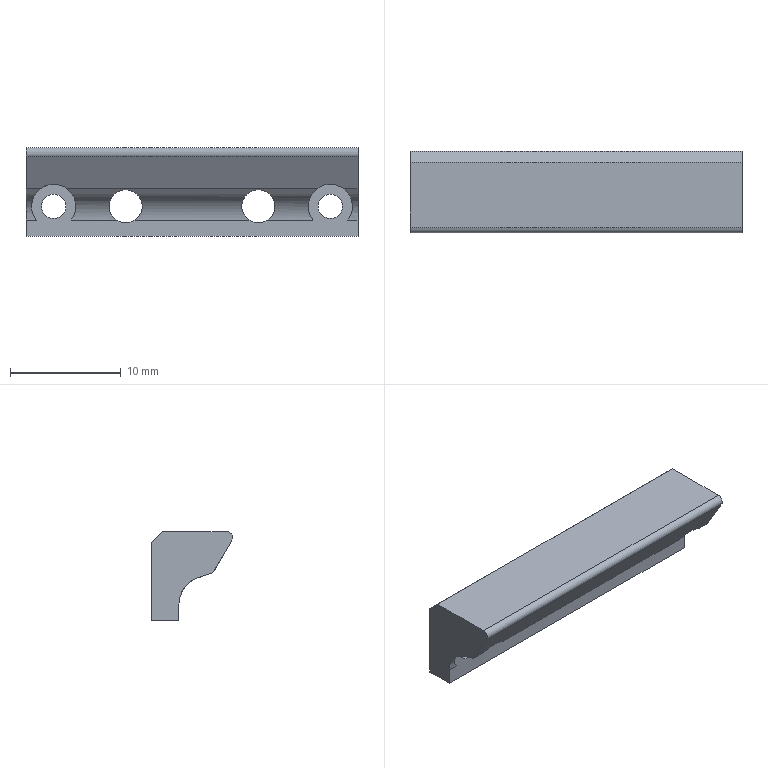Part | SolidWorks | features Cut 3, Extrusion 1, HoleWzd 1 | 1 solid | 28 faces | box 30 x 7.363 x 8 mm | volume 1026 mm3 | cylinder 17 | plane 11 | commonest cylinder face diameters 5 x5 2.2 x4 3 x4 4 x3 1 x1
STEP:
#1=CARTESIAN_POINT('',(-12.5,-2.5,-6.4));
#2=VERTEX_POINT('',#1);
#3=CARTESIAN_POINT('',(-12.5,-2.5,-4.2));
#4=VERTEX_POINT('',#3);
#5=CARTESIAN_POINT('',(-12.5,-2.5,-5.3));
#6=DIRECTION('',(0.,1.,0.));
#7=DIRECTION('',(0.,0.,1.));
#8=AXIS2_PLACEMENT_3D('',#5,#6,#7);
#9=CIRCLE('',#8,1.1);
#10=EDGE_CURVE('',#2,#4,#9,.T.);
#11=ORIENTED_EDGE('',*,*,#10,.T.);
#12=CARTESIAN_POINT('',(-12.5,-5.,-4.2));
#13=VERTEX_POINT('',#12);
#14=CARTESIAN_POINT('',(-12.5,0.,-4.2));
#15=DIRECTION('',(0.,-1.,0.));
#16=VECTOR('',#15,1000.);
#17=LINE('',#14,#16);
#18=EDGE_CURVE('',#4,#13,#17,.T.);
#19=ORIENTED_EDGE('',*,*,#18,.T.);
#20=CARTESIAN_POINT('',(-12.5,-5.,-6.4));
#21=VERTEX_POINT('',#20);
#22=CARTESIAN_POINT('',(-12.5,-5.,-5.3));
#23=DIRECTION('',(0.,-1.,0.));
#24=DIRECTION('',(0.,0.,-1.));
#25=AXIS2_PLACEMENT_3D('',#22,#23,#24);
#26=CIRCLE('',#25,1.1);
#27=EDGE_CURVE('',#13,#21,#26,.T.);
#28=ORIENTED_EDGE('',*,*,#27,.T.);
#29=CARTESIAN_POINT('',(-12.5,0.,-6.4));
#30=DIRECTION('',(0.,-1.,0.));
#31=VECTOR('',#30,1000.);
#32=LINE('',#29,#31);
#33=EDGE_CURVE('',#2,#21,#32,.T.);
#34=ORIENTED_EDGE('',*,*,#33,.F.);
#35=EDGE_LOOP('',(#11,#19,#28,#34));
#36=FACE_OUTER_BOUND('',#35,.T.);
#37=CARTESIAN_POINT('',(-12.5,0.,-5.3));
#38=DIRECTION('',(0.,-1.,0.));
#39=DIRECTION('',(0.,0.,-1.));
#40=AXIS2_PLACEMENT_3D('',#37,#38,#39);
#41=CYLINDRICAL_SURFACE('',#40,1.1);
#42=ADVANCED_FACE('',(#36),#41,.F.);
#43=CARTESIAN_POINT('',(12.5,-2.5,-6.4));
#44=VERTEX_POINT('',#43);
#45=CARTESIAN_POINT('',(12.5,-2.5,-4.2));
#46=VERTEX_POINT('',#45);
#47=CARTESIAN_POINT('',(12.5,-2.5,-5.3));
#48=DIRECTION('',(0.,1.,0.));
#49=DIRECTION('',(0.,0.,1.));
#50=AXIS2_PLACEMENT_3D('',#47,#48,#49);
#51=CIRCLE('',#50,1.1);
#52=EDGE_CURVE('',#44,#46,#51,.T.);
#53=ORIENTED_EDGE('',*,*,#52,.T.);
#54=CARTESIAN_POINT('',(12.5,-5.,-4.2));
#55=VERTEX_POINT('',#54);
#56=CARTESIAN_POINT('',(12.5,0.,-4.2));
#57=DIRECTION('',(0.,-1.,0.));
#58=VECTOR('',#57,1000.);
#59=LINE('',#56,#58);
#60=EDGE_CURVE('',#46,#55,#59,.T.);
#61=ORIENTED_EDGE('',*,*,#60,.T.);
#62=CARTESIAN_POINT('',(12.5,-5.,-6.4));
#63=VERTEX_POINT('',#62);
#64=CARTESIAN_POINT('',(12.5,-5.,-5.3));
#65=DIRECTION('',(0.,-1.,0.));
#66=DIRECTION('',(0.,0.,-1.));
#67=AXIS2_PLACEMENT_3D('',#64,#65,#66);
#68=CIRCLE('',#67,1.1);
#69=EDGE_CURVE('',#55,#63,#68,.T.);
#70=ORIENTED_EDGE('',*,*,#69,.T.);
#71=CARTESIAN_POINT('',(12.5,0.,-6.4));
#72=DIRECTION('',(0.,-1.,0.));
#73=VECTOR('',#72,1000.);
#74=LINE('',#71,#73);
#75=EDGE_CURVE('',#44,#63,#74,.T.);
#76=ORIENTED_EDGE('',*,*,#75,.F.);
#77=EDGE_LOOP('',(#53,#61,#70,#76));
#78=FACE_OUTER_BOUND('',#77,.T.);
#79=CARTESIAN_POINT('',(12.5,0.,-5.3));
#80=DIRECTION('',(0.,-1.,0.));
#81=DIRECTION('',(0.,0.,-1.));
#82=AXIS2_PLACEMENT_3D('',#79,#80,#81);
#83=CYLINDRICAL_SURFACE('',#82,1.1);
#84=ADVANCED_FACE('',(#78),#83,.F.);
#85=CARTESIAN_POINT('',(-12.5,-8.308,-3.3));
#86=VERTEX_POINT('',#85);
#87=CARTESIAN_POINT('',(-11.286,-8.069,-3.71));
#88=VERTEX_POINT('',#87);
#89=CARTESIAN_POINT('',(-12.5,-8.308,-3.3));
#90=CARTESIAN_POINT('',(-12.057,-8.308,-3.3));
#91=CARTESIAN_POINT('',(-11.638,-8.226,-3.442));
#92=CARTESIAN_POINT('',(-11.286,-8.069,-3.71));
#93=(BOUNDED_CURVE()B_SPLINE_CURVE(3,(#89,#90,#91,#92),.UNSPECIFIED.,.F.,.T.)B_SPLINE_CURVE_WITH_KNOTS((4,4),(3.142,3.794),.UNSPECIFIED.)CURVE()GEOMETRIC_REPRESENTATION_ITEM()RATIONAL_B_SPLINE_CURVE((1.,0.9649,0.9649,1.))REPRESENTATION_ITEM(''));
#94=EDGE_CURVE('',#86,#88,#93,.T.);
#95=ORIENTED_EDGE('',*,*,#94,.F.);
#96=CARTESIAN_POINT('',(-12.5,-5.,-3.3));
#97=VERTEX_POINT('',#96);
#98=CARTESIAN_POINT('',(-12.5,-13.192,-3.3));
#99=DIRECTION('',(0.,1.,0.));
#100=VECTOR('',#99,1000.);
#101=LINE('',#98,#100);
#102=EDGE_CURVE('',#86,#97,#101,.T.);
#103=ORIENTED_EDGE('',*,*,#102,.T.);
#104=CARTESIAN_POINT('',(-10.927,-5.,-6.535));
#105=VERTEX_POINT('',#104);
#106=CARTESIAN_POINT('',(-12.5,-5.,-5.3));
#107=DIRECTION('',(0.,-1.,0.));
#108=DIRECTION('',(0.,0.,-1.));
#109=AXIS2_PLACEMENT_3D('',#106,#107,#108);
#110=CIRCLE('',#109,2.);
#111=EDGE_CURVE('',#105,#97,#110,.T.);
#112=ORIENTED_EDGE('',*,*,#111,.F.);
#113=CARTESIAN_POINT('',(-10.854,-6.709,-4.164));
#114=VERTEX_POINT('',#113);
#115=CARTESIAN_POINT('',(-10.854,-6.709,-4.164));
#116=CARTESIAN_POINT('',(-10.796,-6.456,-4.248));
#117=CARTESIAN_POINT('',(-10.722,-6.227,-4.368));
#118=CARTESIAN_POINT('',(-10.624,-5.91,-4.601));
#119=CARTESIAN_POINT('',(-10.593,-5.809,-4.689));
#120=CARTESIAN_POINT('',(-10.542,-5.622,-4.879));
#121=CARTESIAN_POINT('',(-10.522,-5.537,-4.982));
#122=CARTESIAN_POINT('',(-10.499,-5.38,-5.203));
#123=CARTESIAN_POINT('',(-10.496,-5.31,-5.322));
#124=CARTESIAN_POINT('',(-10.514,-5.192,-5.565));
#125=CARTESIAN_POINT('',(-10.534,-5.143,-5.692));
#126=CARTESIAN_POINT('',(-10.636,-5.03,-6.07));
#127=CARTESIAN_POINT('',(-10.757,-5.,-6.319));
#128=CARTESIAN_POINT('',(-10.927,-5.,-6.535));
#129=B_SPLINE_CURVE_WITH_KNOTS('',3,(#115,#116,#117,#118,#119,#120,#121,#122,#123,#124,#125,#126,#127,#128),.UNSPECIFIED.,.F.,.F.,(4,2,2,2,2,2,4),(0.,0.0008052,0.001208,0.00161,0.002013,0.002416,0.003221),.UNSPECIFIED.);
#130=EDGE_CURVE('',#114,#105,#129,.T.);
#131=ORIENTED_EDGE('',*,*,#130,.F.);
#132=CARTESIAN_POINT('',(-11.286,-8.069,-3.71));
#133=CARTESIAN_POINT('',(-11.119,-7.686,-3.838));
#134=CARTESIAN_POINT('',(-10.974,-7.229,-3.99));
#135=CARTESIAN_POINT('',(-10.854,-6.709,-4.164));
#136=(BOUNDED_CURVE()B_SPLINE_CURVE(3,(#132,#133,#134,#135),.UNSPECIFIED.,.F.,.F.)B_SPLINE_CURVE_WITH_KNOTS((4,4),(3.794,4.108),.UNSPECIFIED.)CURVE()GEOMETRIC_REPRESENTATION_ITEM()RATIONAL_B_SPLINE_CURVE((1.,0.9918,0.9918,1.))REPRESENTATION_ITEM(''));
#137=EDGE_CURVE('',#88,#114,#136,.T.);
#138=ORIENTED_EDGE('',*,*,#137,.F.);
#139=EDGE_LOOP('',(#95,#103,#112,#131,#138));
#140=FACE_OUTER_BOUND('',#139,.T.);
#141=CARTESIAN_POINT('',(-12.5,-13.192,-5.3));
#142=DIRECTION('',(0.,1.,0.));
#143=DIRECTION('',(0.,0.,1.));
#144=AXIS2_PLACEMENT_3D('',#141,#142,#143);
#145=CYLINDRICAL_SURFACE('',#144,2.);
#146=ADVANCED_FACE('',(#140),#145,.F.);
#147=CARTESIAN_POINT('',(5.149,-5.,-6.535));
#148=VERTEX_POINT('',#147);
#149=CARTESIAN_POINT('',(6.,-5.,-6.8));
#150=VERTEX_POINT('',#149);
#151=CARTESIAN_POINT('',(6.,-5.,-5.3));
#152=DIRECTION('',(0.,-1.,0.));
#153=DIRECTION('',(0.,0.,-1.));
#154=AXIS2_PLACEMENT_3D('',#151,#152,#153);
#155=CIRCLE('',#154,1.5);
#156=EDGE_CURVE('',#148,#150,#155,.T.);
#157=ORIENTED_EDGE('',*,*,#156,.T.);
#158=CARTESIAN_POINT('',(6.,-2.5,-6.8));
#159=VERTEX_POINT('',#158);
#160=CARTESIAN_POINT('',(6.,-2.5,-6.8));
#161=DIRECTION('',(0.,1.,0.));
#162=VECTOR('',#161,1000.);
#163=LINE('',#160,#162);
#164=EDGE_CURVE('',#150,#159,#163,.T.);
#165=ORIENTED_EDGE('',*,*,#164,.T.);
#166=CARTESIAN_POINT('',(6.,-2.5,-3.8));
#167=VERTEX_POINT('',#166);
#168=CARTESIAN_POINT('',(6.,-2.5,-5.3));
#169=DIRECTION('',(0.,1.,0.));
#170=DIRECTION('',(0.,0.,1.));
#171=AXIS2_PLACEMENT_3D('',#168,#169,#170);
#172=CIRCLE('',#171,1.5);
#173=EDGE_CURVE('',#159,#167,#172,.T.);
#174=ORIENTED_EDGE('',*,*,#173,.T.);
#175=CARTESIAN_POINT('',(6.,-7.8,-3.8));
#176=VERTEX_POINT('',#175);
#177=CARTESIAN_POINT('',(6.,-2.5,-3.8));
#178=DIRECTION('',(0.,1.,0.));
#179=VECTOR('',#178,1000.);
#180=LINE('',#177,#179);
#181=EDGE_CURVE('',#176,#167,#180,.T.);
#182=ORIENTED_EDGE('',*,*,#181,.F.);
#183=CARTESIAN_POINT('',(5.021,-6.709,-4.164));
#184=VERTEX_POINT('',#183);
#185=CARTESIAN_POINT('',(6.,-7.8,-3.8));
#186=CARTESIAN_POINT('',(5.637,-7.8,-3.8));
#187=CARTESIAN_POINT('',(5.296,-7.421,-3.926));
#188=CARTESIAN_POINT('',(5.021,-6.709,-4.164));
#189=(BOUNDED_CURVE()B_SPLINE_CURVE(3,(#185,#186,#187,#188),.UNSPECIFIED.,.F.,.T.)B_SPLINE_CURVE_WITH_KNOTS((4,4),(3.142,3.853),.UNSPECIFIED.)CURVE()GEOMETRIC_REPRESENTATION_ITEM()RATIONAL_B_SPLINE_CURVE((1.,0.9583,0.9583,1.))REPRESENTATION_ITEM(''));
#190=EDGE_CURVE('',#176,#184,#189,.T.);
#191=ORIENTED_EDGE('',*,*,#190,.T.);
#192=CARTESIAN_POINT('',(5.021,-6.709,-4.164));
#193=CARTESIAN_POINT('',(4.922,-6.454,-4.249));
#194=CARTESIAN_POINT('',(4.809,-6.224,-4.369));
#195=CARTESIAN_POINT('',(4.617,-5.793,-4.689));
#196=CARTESIAN_POINT('',(4.538,-5.597,-4.889));
#197=CARTESIAN_POINT('',(4.496,-5.356,-5.241));
#198=CARTESIAN_POINT('',(4.496,-5.286,-5.365));
#199=CARTESIAN_POINT('',(4.53,-5.167,-5.626));
#200=CARTESIAN_POINT('',(4.564,-5.121,-5.755));
#201=CARTESIAN_POINT('',(4.672,-5.052,-6.01));
#202=CARTESIAN_POINT('',(4.745,-5.03,-6.134));
#203=CARTESIAN_POINT('',(4.924,-5.004,-6.354));
#204=CARTESIAN_POINT('',(5.03,-5.,-6.453));
#205=CARTESIAN_POINT('',(5.149,-5.,-6.535));
#206=B_SPLINE_CURVE_WITH_KNOTS('',3,(#192,#193,#194,#195,#196,#197,#198,#199,#200,#201,#202,#203,#204,#205),.UNSPECIFIED.,.F.,.F.,(4,2,2,2,2,2,4),(0.,0.0008481,0.001696,0.00212,0.002544,0.002968,0.003392),.UNSPECIFIED.);
#207=EDGE_CURVE('',#184,#148,#206,.T.);
#208=ORIENTED_EDGE('',*,*,#207,.T.);
#209=EDGE_LOOP('',(#157,#165,#174,#182,#191,#208));
#210=FACE_OUTER_BOUND('',#209,.T.);
#211=CARTESIAN_POINT('',(6.,-2.5,-5.3));
#212=DIRECTION('',(0.,1.,0.));
#213=DIRECTION('',(0.,0.,1.));
#214=AXIS2_PLACEMENT_3D('',#211,#212,#213);
#215=CYLINDRICAL_SURFACE('',#214,1.5);
#216=ADVANCED_FACE('',(#210),#215,.F.);
#217=CARTESIAN_POINT('',(-6.851,-5.,-6.535));
#218=VERTEX_POINT('',#217);
#219=CARTESIAN_POINT('',(-6.,-5.,-6.8));
#220=VERTEX_POINT('',#219);
#221=CARTESIAN_POINT('',(-6.,-5.,-5.3));
#222=DIRECTION('',(0.,-1.,0.));
#223=DIRECTION('',(0.,0.,-1.));
#224=AXIS2_PLACEMENT_3D('',#221,#222,#223);
#225=CIRCLE('',#224,1.5);
#226=EDGE_CURVE('',#218,#220,#225,.T.);
#227=ORIENTED_EDGE('',*,*,#226,.T.);
#228=CARTESIAN_POINT('',(-6.,-2.5,-6.8));
#229=VERTEX_POINT('',#228);
#230=CARTESIAN_POINT('',(-6.,-2.5,-6.8));
#231=DIRECTION('',(0.,1.,0.));
#232=VECTOR('',#231,1000.);
#233=LINE('',#230,#232);
#234=EDGE_CURVE('',#220,#229,#233,.T.);
#235=ORIENTED_EDGE('',*,*,#234,.T.);
#236=CARTESIAN_POINT('',(-6.,-2.5,-3.8));
#237=VERTEX_POINT('',#236);
#238=CARTESIAN_POINT('',(-6.,-2.5,-5.3));
#239=DIRECTION('',(0.,1.,0.));
#240=DIRECTION('',(0.,0.,1.));
#241=AXIS2_PLACEMENT_3D('',#238,#239,#240);
#242=CIRCLE('',#241,1.5);
#243=EDGE_CURVE('',#229,#237,#242,.T.);
#244=ORIENTED_EDGE('',*,*,#243,.T.);
#245=CARTESIAN_POINT('',(-6.,-7.8,-3.8));
#246=VERTEX_POINT('',#245);
#247=CARTESIAN_POINT('',(-6.,-2.5,-3.8));
#248=DIRECTION('',(0.,1.,0.));
#249=VECTOR('',#248,1000.);
#250=LINE('',#247,#249);
#251=EDGE_CURVE('',#246,#237,#250,.T.);
#252=ORIENTED_EDGE('',*,*,#251,.F.);
#253=CARTESIAN_POINT('',(-6.979,-6.709,-4.164));
#254=VERTEX_POINT('',#253);
#255=CARTESIAN_POINT('',(-6.,-7.8,-3.8));
#256=CARTESIAN_POINT('',(-6.363,-7.8,-3.8));
#257=CARTESIAN_POINT('',(-6.704,-7.421,-3.926));
#258=CARTESIAN_POINT('',(-6.979,-6.709,-4.164));
#259=(BOUNDED_CURVE()B_SPLINE_CURVE(3,(#255,#256,#257,#258),.UNSPECIFIED.,.F.,.F.)B_SPLINE_CURVE_WITH_KNOTS((4,4),(3.142,3.853),.UNSPECIFIED.)CURVE()GEOMETRIC_REPRESENTATION_ITEM()RATIONAL_B_SPLINE_CURVE((1.,0.9583,0.9583,1.))REPRESENTATION_ITEM(''));
#260=EDGE_CURVE('',#246,#254,#259,.T.);
#261=ORIENTED_EDGE('',*,*,#260,.T.);
#262=CARTESIAN_POINT('',(-6.979,-6.709,-4.164));
#263=CARTESIAN_POINT('',(-7.078,-6.454,-4.249));
#264=CARTESIAN_POINT('',(-7.191,-6.224,-4.369));
#265=CARTESIAN_POINT('',(-7.383,-5.793,-4.689));
#266=CARTESIAN_POINT('',(-7.462,-5.597,-4.889));
#267=CARTESIAN_POINT('',(-7.504,-5.356,-5.241));
#268=CARTESIAN_POINT('',(-7.504,-5.286,-5.365));
#269=CARTESIAN_POINT('',(-7.47,-5.167,-5.626));
#270=CARTESIAN_POINT('',(-7.436,-5.121,-5.755));
#271=CARTESIAN_POINT('',(-7.328,-5.052,-6.01));
#272=CARTESIAN_POINT('',(-7.255,-5.03,-6.134));
#273=CARTESIAN_POINT('',(-7.076,-5.004,-6.354));
#274=CARTESIAN_POINT('',(-6.97,-5.,-6.453));
#275=CARTESIAN_POINT('',(-6.851,-5.,-6.535));
#276=B_SPLINE_CURVE_WITH_KNOTS('',3,(#262,#263,#264,#265,#266,#267,#268,#269,#270,#271,#272,#273,#274,#275),.UNSPECIFIED.,.F.,.F.,(4,2,2,2,2,2,4),(0.,0.0008481,0.001696,0.00212,0.002544,0.002968,0.003392),.UNSPECIFIED.);
#277=EDGE_CURVE('',#254,#218,#276,.T.);
#278=ORIENTED_EDGE('',*,*,#277,.T.);
#279=EDGE_LOOP('',(#227,#235,#244,#252,#261,#278));
#280=FACE_OUTER_BOUND('',#279,.T.);
#281=CARTESIAN_POINT('',(-6.,-2.5,-5.3));
#282=DIRECTION('',(0.,1.,0.));
#283=DIRECTION('',(0.,0.,1.));
#284=AXIS2_PLACEMENT_3D('',#281,#282,#283);
#285=CYLINDRICAL_SURFACE('',#284,1.5);
#286=ADVANCED_FACE('',(#280),#285,.F.);
#287=CARTESIAN_POINT('',(-25.872,-6.709,-4.164));
#288=DIRECTION('',(1.,0.,0.));
#289=VECTOR('',#288,1000.);
#290=LINE('',#287,#289);
#291=EDGE_CURVE('',#114,#254,#290,.T.);
#292=ORIENTED_EDGE('',*,*,#291,.F.);
#293=ORIENTED_EDGE('',*,*,#130,.T.);
#294=CARTESIAN_POINT('',(-25.872,-5.,-6.535));
#295=DIRECTION('',(1.,0.,0.));
#296=VECTOR('',#295,1000.);
#297=LINE('',#294,#296);
#298=EDGE_CURVE('',#105,#218,#297,.T.);
#299=ORIENTED_EDGE('',*,*,#298,.T.);
#300=ORIENTED_EDGE('',*,*,#277,.F.);
#301=EDGE_LOOP('',(#292,#293,#299,#300));
#302=FACE_OUTER_BOUND('',#301,.T.);
#303=CARTESIAN_POINT('',(-25.872,-7.5,-6.535));
#304=DIRECTION('',(1.,0.,0.));
#305=DIRECTION('',(0.,0.,-1.));
#306=AXIS2_PLACEMENT_3D('',#303,#304,#305);
#307=CYLINDRICAL_SURFACE('',#306,2.5);
#308=ADVANCED_FACE('',(#302),#307,.F.);
#309=CARTESIAN_POINT('',(-15.,-5.,-6.535));
#310=VERTEX_POINT('',#309);
#311=CARTESIAN_POINT('',(-14.073,-5.,-6.535));
#312=VERTEX_POINT('',#311);
#313=CARTESIAN_POINT('',(-25.872,-5.,-6.535));
#314=DIRECTION('',(1.,0.,0.));
#315=VECTOR('',#314,1000.);
#316=LINE('',#313,#315);
#317=EDGE_CURVE('',#310,#312,#316,.T.);
#318=ORIENTED_EDGE('',*,*,#317,.T.);
#319=CARTESIAN_POINT('',(-14.146,-6.709,-4.164));
#320=VERTEX_POINT('',#319);
#321=CARTESIAN_POINT('',(-14.073,-5.,-6.535));
#322=CARTESIAN_POINT('',(-14.158,-5.,-6.427));
#323=CARTESIAN_POINT('',(-14.23,-5.007,-6.313));
#324=CARTESIAN_POINT('',(-14.35,-5.04,-6.072));
#325=CARTESIAN_POINT('',(-14.398,-5.067,-5.945));
#326=CARTESIAN_POINT('',(-14.465,-5.142,-5.694));
#327=CARTESIAN_POINT('',(-14.486,-5.191,-5.568));
#328=CARTESIAN_POINT('',(-14.504,-5.309,-5.323));
#329=CARTESIAN_POINT('',(-14.501,-5.378,-5.206));
#330=CARTESIAN_POINT('',(-14.467,-5.613,-4.873));
#331=CARTESIAN_POINT('',(-14.41,-5.8,-4.683));
#332=CARTESIAN_POINT('',(-14.278,-6.226,-4.368));
#333=CARTESIAN_POINT('',(-14.204,-6.456,-4.248));
#334=CARTESIAN_POINT('',(-14.146,-6.709,-4.164));
#335=B_SPLINE_CURVE_WITH_KNOTS('',3,(#321,#322,#323,#324,#325,#326,#327,#328,#329,#330,#331,#332,#333,#334),.UNSPECIFIED.,.F.,.F.,(4,2,2,2,2,2,4),(0.,0.0004056,0.0008113,0.001217,0.001623,0.002434,0.003245),.UNSPECIFIED.);
#336=EDGE_CURVE('',#312,#320,#335,.T.);
#337=ORIENTED_EDGE('',*,*,#336,.T.);
#338=CARTESIAN_POINT('',(-15.,-6.709,-4.164));
#339=VERTEX_POINT('',#338);
#340=CARTESIAN_POINT('',(-25.872,-6.709,-4.164));
#341=DIRECTION('',(1.,0.,0.));
#342=VECTOR('',#341,1000.);
#343=LINE('',#340,#342);
#344=EDGE_CURVE('',#339,#320,#343,.T.);
#345=ORIENTED_EDGE('',*,*,#344,.F.);
#346=CARTESIAN_POINT('',(-15.,-7.5,-6.535));
#347=DIRECTION('',(1.,0.,0.));
#348=DIRECTION('',(0.,0.,-1.));
#349=AXIS2_PLACEMENT_3D('',#346,#347,#348);
#350=CIRCLE('',#349,2.5);
#351=EDGE_CURVE('',#310,#339,#350,.T.);
#352=ORIENTED_EDGE('',*,*,#351,.F.);
#353=EDGE_LOOP('',(#318,#337,#345,#352));
#354=FACE_OUTER_BOUND('',#353,.T.);
#355=CARTESIAN_POINT('',(-25.872,-7.5,-6.535));
#356=DIRECTION('',(1.,0.,0.));
#357=DIRECTION('',(0.,0.,-1.));
#358=AXIS2_PLACEMENT_3D('',#355,#356,#357);
#359=CYLINDRICAL_SURFACE('',#358,2.5);
#360=ADVANCED_FACE('',(#354),#359,.F.);
#361=ORIENTED_EDGE('',*,*,#344,.T.);
#362=CARTESIAN_POINT('',(-13.714,-8.069,-3.71));
#363=VERTEX_POINT('',#362);
#364=CARTESIAN_POINT('',(-14.146,-6.709,-4.164));
#365=CARTESIAN_POINT('',(-14.026,-7.229,-3.99));
#366=CARTESIAN_POINT('',(-13.881,-7.686,-3.838));
#367=CARTESIAN_POINT('',(-13.714,-8.069,-3.71));
#368=(BOUNDED_CURVE()B_SPLINE_CURVE(3,(#364,#365,#366,#367),.UNSPECIFIED.,.F.,.F.)B_SPLINE_CURVE_WITH_KNOTS((4,4),(2.175,2.49),.UNSPECIFIED.)CURVE()GEOMETRIC_REPRESENTATION_ITEM()RATIONAL_B_SPLINE_CURVE((1.,0.9918,0.9918,1.))REPRESENTATION_ITEM(''));
#369=EDGE_CURVE('',#320,#363,#368,.T.);
#370=ORIENTED_EDGE('',*,*,#369,.T.);
#371=CARTESIAN_POINT('',(-15.,-8.069,-3.71));
#372=VERTEX_POINT('',#371);
#373=CARTESIAN_POINT('',(-25.872,-8.069,-3.71));
#374=DIRECTION('',(1.,0.,0.));
#375=VECTOR('',#374,1000.);
#376=LINE('',#373,#375);
#377=EDGE_CURVE('',#372,#363,#376,.T.);
#378=ORIENTED_EDGE('',*,*,#377,.F.);
#379=CARTESIAN_POINT('',(-15.,-4.2,-5.));
#380=DIRECTION('',(0.,0.9487,-0.3162));
#381=VECTOR('',#380,1000.);
#382=LINE('',#379,#381);
#383=EDGE_CURVE('',#372,#339,#382,.T.);
#384=ORIENTED_EDGE('',*,*,#383,.T.);
#385=EDGE_LOOP('',(#361,#370,#378,#384));
#386=FACE_OUTER_BOUND('',#385,.T.);
#387=CARTESIAN_POINT('',(-25.872,-8.069,-3.71));
#388=DIRECTION('',(0.,-0.3162,-0.9487));
#389=DIRECTION('',(0.,0.9487,-0.3162));
#390=AXIS2_PLACEMENT_3D('',#387,#388,#389);
#391=PLANE('',#390);
#392=ADVANCED_FACE('',(#386),#391,.T.);
#393=CARTESIAN_POINT('',(11.286,-8.069,-3.71));
#394=VERTEX_POINT('',#393);
#395=CARTESIAN_POINT('',(-25.872,-8.069,-3.71));
#396=DIRECTION('',(1.,0.,0.));
#397=VECTOR('',#396,1000.);
#398=LINE('',#395,#397);
#399=EDGE_CURVE('',#88,#394,#398,.T.);
#400=ORIENTED_EDGE('',*,*,#399,.F.);
#401=ORIENTED_EDGE('',*,*,#137,.T.);
#402=ORIENTED_EDGE('',*,*,#291,.T.);
#403=ORIENTED_EDGE('',*,*,#260,.F.);
#404=CARTESIAN_POINT('',(-5.021,-6.709,-4.164));
#405=VERTEX_POINT('',#404);
#406=CARTESIAN_POINT('',(-5.021,-6.709,-4.164));
#407=CARTESIAN_POINT('',(-5.296,-7.421,-3.926));
#408=CARTESIAN_POINT('',(-5.637,-7.8,-3.8));
#409=CARTESIAN_POINT('',(-6.,-7.8,-3.8));
#410=(BOUNDED_CURVE()B_SPLINE_CURVE(3,(#406,#407,#408,#409),.UNSPECIFIED.,.F.,.T.)B_SPLINE_CURVE_WITH_KNOTS((4,4),(2.431,3.142),.UNSPECIFIED.)CURVE()GEOMETRIC_REPRESENTATION_ITEM()RATIONAL_B_SPLINE_CURVE((1.,0.9583,0.9583,1.))REPRESENTATION_ITEM(''));
#411=EDGE_CURVE('',#405,#246,#410,.T.);
#412=ORIENTED_EDGE('',*,*,#411,.F.);
#413=CARTESIAN_POINT('',(-25.872,-6.709,-4.164));
#414=DIRECTION('',(1.,0.,0.));
#415=VECTOR('',#414,1000.);
#416=LINE('',#413,#415);
#417=EDGE_CURVE('',#405,#184,#416,.T.);
#418=ORIENTED_EDGE('',*,*,#417,.T.);
#419=ORIENTED_EDGE('',*,*,#190,.F.);
#420=CARTESIAN_POINT('',(6.979,-6.709,-4.164));
#421=VERTEX_POINT('',#420);
#422=CARTESIAN_POINT('',(6.979,-6.709,-4.164));
#423=CARTESIAN_POINT('',(6.704,-7.421,-3.926));
#424=CARTESIAN_POINT('',(6.363,-7.8,-3.8));
#425=CARTESIAN_POINT('',(6.,-7.8,-3.8));
#426=(BOUNDED_CURVE()B_SPLINE_CURVE(3,(#422,#423,#424,#425),.UNSPECIFIED.,.F.,.F.)B_SPLINE_CURVE_WITH_KNOTS((4,4),(2.431,3.142),.UNSPECIFIED.)CURVE()GEOMETRIC_REPRESENTATION_ITEM()RATIONAL_B_SPLINE_CURVE((1.,0.9583,0.9583,1.))REPRESENTATION_ITEM(''));
#427=EDGE_CURVE('',#421,#176,#426,.T.);
#428=ORIENTED_EDGE('',*,*,#427,.F.);
#429=CARTESIAN_POINT('',(10.854,-6.709,-4.164));
#430=VERTEX_POINT('',#429);
#431=CARTESIAN_POINT('',(-25.872,-6.709,-4.164));
#432=DIRECTION('',(1.,0.,0.));
#433=VECTOR('',#432,1000.);
#434=LINE('',#431,#433);
#435=EDGE_CURVE('',#421,#430,#434,.T.);
#436=ORIENTED_EDGE('',*,*,#435,.T.);
#437=CARTESIAN_POINT('',(10.854,-6.709,-4.164));
#438=CARTESIAN_POINT('',(10.974,-7.229,-3.99));
#439=CARTESIAN_POINT('',(11.119,-7.686,-3.838));
#440=CARTESIAN_POINT('',(11.286,-8.069,-3.71));
#441=(BOUNDED_CURVE()B_SPLINE_CURVE(3,(#437,#438,#439,#440),.UNSPECIFIED.,.F.,.T.)B_SPLINE_CURVE_WITH_KNOTS((4,4),(5.317,5.631),.UNSPECIFIED.)CURVE()GEOMETRIC_REPRESENTATION_ITEM()RATIONAL_B_SPLINE_CURVE((1.,0.9918,0.9918,1.))REPRESENTATION_ITEM(''));
#442=EDGE_CURVE('',#430,#394,#441,.T.);
#443=ORIENTED_EDGE('',*,*,#442,.T.);
#444=EDGE_LOOP('',(#400,#401,#402,#403,#412,#418,#419,#428,#436,#443));
#445=FACE_OUTER_BOUND('',#444,.T.);
#446=CARTESIAN_POINT('',(-25.872,-8.069,-3.71));
#447=DIRECTION('',(0.,-0.3162,-0.9487));
#448=DIRECTION('',(0.,0.9487,-0.3162));
#449=AXIS2_PLACEMENT_3D('',#446,#447,#448);
#450=PLANE('',#449);
#451=ADVANCED_FACE('',(#445),#450,.T.);
#452=CARTESIAN_POINT('',(14.146,-6.709,-4.164));
#453=VERTEX_POINT('',#452);
#454=CARTESIAN_POINT('',(15.,-6.709,-4.164));
#455=VERTEX_POINT('',#454);
#456=CARTESIAN_POINT('',(-25.872,-6.709,-4.164));
#457=DIRECTION('',(1.,0.,0.));
#458=VECTOR('',#457,1000.);
#459=LINE('',#456,#458);
#460=EDGE_CURVE('',#453,#455,#459,.T.);
#461=ORIENTED_EDGE('',*,*,#460,.F.);
#462=CARTESIAN_POINT('',(14.073,-5.,-6.535));
#463=VERTEX_POINT('',#462);
#464=CARTESIAN_POINT('',(14.146,-6.709,-4.164));
#465=CARTESIAN_POINT('',(14.204,-6.456,-4.248));
#466=CARTESIAN_POINT('',(14.278,-6.227,-4.368));
#467=CARTESIAN_POINT('',(14.376,-5.91,-4.601));
#468=CARTESIAN_POINT('',(14.407,-5.809,-4.689));
#469=CARTESIAN_POINT('',(14.458,-5.622,-4.879));
#470=CARTESIAN_POINT('',(14.478,-5.537,-4.982));
#471=CARTESIAN_POINT('',(14.501,-5.38,-5.203));
#472=CARTESIAN_POINT('',(14.504,-5.31,-5.322));
#473=CARTESIAN_POINT('',(14.486,-5.192,-5.565));
#474=CARTESIAN_POINT('',(14.466,-5.143,-5.692));
#475=CARTESIAN_POINT('',(14.364,-5.03,-6.07));
#476=CARTESIAN_POINT('',(14.243,-5.,-6.319));
#477=CARTESIAN_POINT('',(14.073,-5.,-6.535));
#478=B_SPLINE_CURVE_WITH_KNOTS('',3,(#464,#465,#466,#467,#468,#469,#470,#471,#472,#473,#474,#475,#476,#477),.UNSPECIFIED.,.F.,.F.,(4,2,2,2,2,2,4),(0.,0.0008052,0.001208,0.00161,0.002013,0.002416,0.003221),.UNSPECIFIED.);
#479=EDGE_CURVE('',#453,#463,#478,.T.);
#480=ORIENTED_EDGE('',*,*,#479,.T.);
#481=CARTESIAN_POINT('',(15.,-5.,-6.535));
#482=VERTEX_POINT('',#481);
#483=CARTESIAN_POINT('',(-25.872,-5.,-6.535));
#484=DIRECTION('',(1.,0.,0.));
#485=VECTOR('',#484,1000.);
#486=LINE('',#483,#485);
#487=EDGE_CURVE('',#463,#482,#486,.T.);
#488=ORIENTED_EDGE('',*,*,#487,.T.);
#489=CARTESIAN_POINT('',(15.,-7.5,-6.535));
#490=DIRECTION('',(-1.,0.,0.));
#491=DIRECTION('',(0.,0.,-1.));
#492=AXIS2_PLACEMENT_3D('',#489,#490,#491);
#493=CIRCLE('',#492,2.5);
#494=EDGE_CURVE('',#455,#482,#493,.T.);
#495=ORIENTED_EDGE('',*,*,#494,.F.);
#496=EDGE_LOOP('',(#461,#480,#488,#495));
#497=FACE_OUTER_BOUND('',#496,.T.);
#498=CARTESIAN_POINT('',(-25.872,-7.5,-6.535));
#499=DIRECTION('',(1.,0.,0.));
#500=DIRECTION('',(0.,0.,-1.));
#501=AXIS2_PLACEMENT_3D('',#498,#499,#500);
#502=CYLINDRICAL_SURFACE('',#501,2.5);
#503=ADVANCED_FACE('',(#497),#502,.F.);
#504=CARTESIAN_POINT('',(6.851,-5.,-6.535));
#505=VERTEX_POINT('',#504);
#506=CARTESIAN_POINT('',(10.927,-5.,-6.535));
#507=VERTEX_POINT('',#506);
#508=CARTESIAN_POINT('',(-25.872,-5.,-6.535));
#509=DIRECTION('',(1.,0.,0.));
#510=VECTOR('',#509,1000.);
#511=LINE('',#508,#510);
#512=EDGE_CURVE('',#505,#507,#511,.T.);
#513=ORIENTED_EDGE('',*,*,#512,.T.);
#514=CARTESIAN_POINT('',(10.927,-5.,-6.535));
#515=CARTESIAN_POINT('',(10.842,-5.,-6.427));
#516=CARTESIAN_POINT('',(10.77,-5.007,-6.313));
#517=CARTESIAN_POINT('',(10.65,-5.04,-6.072));
#518=CARTESIAN_POINT('',(10.602,-5.067,-5.945));
#519=CARTESIAN_POINT('',(10.535,-5.142,-5.694));
#520=CARTESIAN_POINT('',(10.514,-5.191,-5.568));
#521=CARTESIAN_POINT('',(10.496,-5.309,-5.323));
#522=CARTESIAN_POINT('',(10.499,-5.378,-5.206));
#523=CARTESIAN_POINT('',(10.533,-5.613,-4.873));
#524=CARTESIAN_POINT('',(10.59,-5.8,-4.683));
#525=CARTESIAN_POINT('',(10.722,-6.226,-4.368));
#526=CARTESIAN_POINT('',(10.796,-6.456,-4.248));
#527=CARTESIAN_POINT('',(10.854,-6.709,-4.164));
#528=B_SPLINE_CURVE_WITH_KNOTS('',3,(#514,#515,#516,#517,#518,#519,#520,#521,#522,#523,#524,#525,#526,#527),.UNSPECIFIED.,.F.,.F.,(4,2,2,2,2,2,4),(0.,0.0004056,0.0008113,0.001217,0.001623,0.002434,0.003245),.UNSPECIFIED.);
#529=EDGE_CURVE('',#507,#430,#528,.T.);
#530=ORIENTED_EDGE('',*,*,#529,.T.);
#531=ORIENTED_EDGE('',*,*,#435,.F.);
#532=CARTESIAN_POINT('',(6.851,-5.,-6.535));
#533=CARTESIAN_POINT('',(6.97,-5.,-6.454));
#534=CARTESIAN_POINT('',(7.074,-5.004,-6.357));
#535=CARTESIAN_POINT('',(7.254,-5.03,-6.135));
#536=CARTESIAN_POINT('',(7.327,-5.051,-6.014));
#537=CARTESIAN_POINT('',(7.435,-5.12,-5.759));
#538=CARTESIAN_POINT('',(7.47,-5.167,-5.626));
#539=CARTESIAN_POINT('',(7.504,-5.284,-5.368));
#540=CARTESIAN_POINT('',(7.504,-5.356,-5.242));
#541=CARTESIAN_POINT('',(7.476,-5.516,-5.008));
#542=CARTESIAN_POINT('',(7.449,-5.606,-4.898));
#543=CARTESIAN_POINT('',(7.379,-5.797,-4.7));
#544=CARTESIAN_POINT('',(7.336,-5.898,-4.611));
#545=CARTESIAN_POINT('',(7.191,-6.223,-4.369));
#546=CARTESIAN_POINT('',(7.078,-6.454,-4.249));
#547=CARTESIAN_POINT('',(6.979,-6.709,-4.164));
#548=B_SPLINE_CURVE_WITH_KNOTS('',3,(#532,#533,#534,#535,#536,#537,#538,#539,#540,#541,#542,#543,#544,#545,#546,#547),.UNSPECIFIED.,.F.,.F.,(4,2,2,2,2,2,2,4),(0.,0.0004263,0.0008525,0.001279,0.001705,0.002131,0.002558,0.00341),.UNSPECIFIED.);
#549=EDGE_CURVE('',#505,#421,#548,.T.);
#550=ORIENTED_EDGE('',*,*,#549,.F.);
#551=EDGE_LOOP('',(#513,#530,#531,#550));
#552=FACE_OUTER_BOUND('',#551,.T.);
#553=CARTESIAN_POINT('',(-25.872,-7.5,-6.535));
#554=DIRECTION('',(1.,0.,0.));
#555=DIRECTION('',(0.,0.,-1.));
#556=AXIS2_PLACEMENT_3D('',#553,#554,#555);
#557=CYLINDRICAL_SURFACE('',#556,2.5);
#558=ADVANCED_FACE('',(#552),#557,.F.);
#559=CARTESIAN_POINT('',(13.714,-8.069,-3.71));
#560=VERTEX_POINT('',#559);
#561=CARTESIAN_POINT('',(15.,-8.069,-3.71));
#562=VERTEX_POINT('',#561);
#563=CARTESIAN_POINT('',(-25.872,-8.069,-3.71));
#564=DIRECTION('',(1.,0.,0.));
#565=VECTOR('',#564,1000.);
#566=LINE('',#563,#565);
#567=EDGE_CURVE('',#560,#562,#566,.T.);
#568=ORIENTED_EDGE('',*,*,#567,.F.);
#569=CARTESIAN_POINT('',(13.714,-8.069,-3.71));
#570=CARTESIAN_POINT('',(13.881,-7.686,-3.838));
#571=CARTESIAN_POINT('',(14.026,-7.229,-3.99));
#572=CARTESIAN_POINT('',(14.146,-6.709,-4.164));
#573=(BOUNDED_CURVE()B_SPLINE_CURVE(3,(#569,#570,#571,#572),.UNSPECIFIED.,.F.,.F.)B_SPLINE_CURVE_WITH_KNOTS((4,4),(0.6521,0.9664),.UNSPECIFIED.)CURVE()GEOMETRIC_REPRESENTATION_ITEM()RATIONAL_B_SPLINE_CURVE((1.,0.9918,0.9918,1.))REPRESENTATION_ITEM(''));
#574=EDGE_CURVE('',#560,#453,#573,.T.);
#575=ORIENTED_EDGE('',*,*,#574,.T.);
#576=ORIENTED_EDGE('',*,*,#460,.T.);
#577=CARTESIAN_POINT('',(15.,-8.069,-3.71));
#578=DIRECTION('',(0.,0.9487,-0.3162));
#579=VECTOR('',#578,1000.);
#580=LINE('',#577,#579);
#581=EDGE_CURVE('',#562,#455,#580,.T.);
#582=ORIENTED_EDGE('',*,*,#581,.F.);
#583=EDGE_LOOP('',(#568,#575,#576,#582));
#584=FACE_OUTER_BOUND('',#583,.T.);
#585=CARTESIAN_POINT('',(-25.872,-8.069,-3.71));
#586=DIRECTION('',(0.,-0.3162,-0.9487));
#587=DIRECTION('',(0.,0.9487,-0.3162));
#588=AXIS2_PLACEMENT_3D('',#585,#586,#587);
#589=PLANE('',#588);
#590=ADVANCED_FACE('',(#584),#589,.T.);
#591=ORIENTED_EDGE('',*,*,#207,.F.);
#592=ORIENTED_EDGE('',*,*,#417,.F.);
#593=CARTESIAN_POINT('',(-5.149,-5.,-6.535));
#594=VERTEX_POINT('',#593);
#595=CARTESIAN_POINT('',(-5.149,-5.,-6.535));
#596=CARTESIAN_POINT('',(-5.03,-5.,-6.454));
#597=CARTESIAN_POINT('',(-4.926,-5.004,-6.357));
#598=CARTESIAN_POINT('',(-4.746,-5.03,-6.135));
#599=CARTESIAN_POINT('',(-4.673,-5.051,-6.014));
#600=CARTESIAN_POINT('',(-4.565,-5.12,-5.759));
#601=CARTESIAN_POINT('',(-4.53,-5.167,-5.626));
#602=CARTESIAN_POINT('',(-4.496,-5.284,-5.368));
#603=CARTESIAN_POINT('',(-4.496,-5.356,-5.242));
#604=CARTESIAN_POINT('',(-4.524,-5.516,-5.008));
#605=CARTESIAN_POINT('',(-4.551,-5.606,-4.898));
#606=CARTESIAN_POINT('',(-4.621,-5.797,-4.7));
#607=CARTESIAN_POINT('',(-4.664,-5.898,-4.611));
#608=CARTESIAN_POINT('',(-4.809,-6.223,-4.369));
#609=CARTESIAN_POINT('',(-4.922,-6.454,-4.249));
#610=CARTESIAN_POINT('',(-5.021,-6.709,-4.164));
#611=B_SPLINE_CURVE_WITH_KNOTS('',3,(#595,#596,#597,#598,#599,#600,#601,#602,#603,#604,#605,#606,#607,#608,#609,#610),.UNSPECIFIED.,.F.,.F.,(4,2,2,2,2,2,2,4),(0.,0.0004263,0.0008525,0.001279,0.001705,0.002131,0.002558,0.00341),.UNSPECIFIED.);
#612=EDGE_CURVE('',#594,#405,#611,.T.);
#613=ORIENTED_EDGE('',*,*,#612,.F.);
#614=CARTESIAN_POINT('',(-25.872,-5.,-6.535));
#615=DIRECTION('',(1.,0.,0.));
#616=VECTOR('',#615,1000.);
#617=LINE('',#614,#616);
#618=EDGE_CURVE('',#594,#148,#617,.T.);
#619=ORIENTED_EDGE('',*,*,#618,.T.);
#620=EDGE_LOOP('',(#591,#592,#613,#619));
#621=FACE_OUTER_BOUND('',#620,.T.);
#622=CARTESIAN_POINT('',(-25.872,-7.5,-6.535));
#623=DIRECTION('',(1.,0.,0.));
#624=DIRECTION('',(0.,0.,-1.));
#625=AXIS2_PLACEMENT_3D('',#622,#623,#624);
#626=CYLINDRICAL_SURFACE('',#625,2.5);
#627=ADVANCED_FACE('',(#621),#626,.F.);
#628=CARTESIAN_POINT('',(-15.,-9.363,0.));
#629=VERTEX_POINT('',#628);
#630=CARTESIAN_POINT('',(-15.,-3.5,0.));
#631=VERTEX_POINT('',#630);
#632=CARTESIAN_POINT('',(-15.,-8.591,0.));
#633=DIRECTION('',(0.,1.,0.));
#634=VECTOR('',#633,1000.);
#635=LINE('',#632,#634);
#636=EDGE_CURVE('',#629,#631,#635,.T.);
#637=ORIENTED_EDGE('',*,*,#636,.F.);
#638=CARTESIAN_POINT('',(15.,-9.363,0.));
#639=VERTEX_POINT('',#638);
#640=CARTESIAN_POINT('',(-25.872,-9.363,0.));
#641=DIRECTION('',(1.,0.,0.));
#642=VECTOR('',#641,1000.);
#643=LINE('',#640,#642);
#644=EDGE_CURVE('',#629,#639,#643,.T.);
#645=ORIENTED_EDGE('',*,*,#644,.T.);
#646=CARTESIAN_POINT('',(15.,-3.5,0.));
#647=VERTEX_POINT('',#646);
#648=CARTESIAN_POINT('',(15.,-3.5,0.));
#649=DIRECTION('',(0.,-1.,0.));
#650=VECTOR('',#649,1000.);
#651=LINE('',#648,#650);
#652=EDGE_CURVE('',#647,#639,#651,.T.);
#653=ORIENTED_EDGE('',*,*,#652,.F.);
#654=CARTESIAN_POINT('',(-25.872,-3.5,0.));
#655=DIRECTION('',(1.,0.,0.));
#656=VECTOR('',#655,1000.);
#657=LINE('',#654,#656);
#658=EDGE_CURVE('',#631,#647,#657,.T.);
#659=ORIENTED_EDGE('',*,*,#658,.F.);
#660=EDGE_LOOP('',(#637,#645,#653,#659));
#661=FACE_OUTER_BOUND('',#660,.T.);
#662=CARTESIAN_POINT('',(-25.872,-3.5,0.));
#663=DIRECTION('',(0.,0.,1.));
#664=DIRECTION('',(0.,-1.,0.));
#665=AXIS2_PLACEMENT_3D('',#662,#663,#664);
#666=PLANE('',#665);
#667=ADVANCED_FACE('',(#661),#666,.T.);
#668=CARTESIAN_POINT('',(-15.,-2.5,-1.));
#669=VERTEX_POINT('',#668);
#670=CARTESIAN_POINT('',(-15.,-3.5,0.));
#671=DIRECTION('',(0.,0.7071,-0.7071));
#672=VECTOR('',#671,1000.);
#673=LINE('',#670,#672);
#674=EDGE_CURVE('',#631,#669,#673,.T.);
#675=ORIENTED_EDGE('',*,*,#674,.F.);
#676=ORIENTED_EDGE('',*,*,#658,.T.);
#677=CARTESIAN_POINT('',(15.,-2.5,-1.));
#678=VERTEX_POINT('',#677);
#679=CARTESIAN_POINT('',(15.,-3.5,0.));
#680=DIRECTION('',(0.,-0.7071,0.7071));
#681=VECTOR('',#680,1000.);
#682=LINE('',#679,#681);
#683=EDGE_CURVE('',#678,#647,#682,.T.);
#684=ORIENTED_EDGE('',*,*,#683,.F.);
#685=CARTESIAN_POINT('',(-25.872,-2.5,-1.));
#686=DIRECTION('',(1.,0.,0.));
#687=VECTOR('',#686,1000.);
#688=LINE('',#685,#687);
#689=EDGE_CURVE('',#669,#678,#688,.T.);
#690=ORIENTED_EDGE('',*,*,#689,.F.);
#691=EDGE_LOOP('',(#675,#676,#684,#690));
#692=FACE_OUTER_BOUND('',#691,.T.);
#693=CARTESIAN_POINT('',(-25.872,-3.5,0.));
#694=DIRECTION('',(0.,0.7071,0.7071));
#695=DIRECTION('',(0.,-0.7071,0.7071));
#696=AXIS2_PLACEMENT_3D('',#693,#694,#695);
#697=PLANE('',#696);
#698=ADVANCED_FACE('',(#692),#697,.T.);
#699=ORIENTED_EDGE('',*,*,#10,.F.);
#700=CARTESIAN_POINT('',(-12.5,-2.5,-5.3));
#701=DIRECTION('',(0.,1.,0.));
#702=DIRECTION('',(0.,0.,1.));
#703=AXIS2_PLACEMENT_3D('',#700,#701,#702);
#704=CIRCLE('',#703,1.1);
#705=EDGE_CURVE('',#4,#2,#704,.T.);
#706=ORIENTED_EDGE('',*,*,#705,.F.);
#707=EDGE_LOOP('',(#699,#706));
#708=FACE_BOUND('',#707,.T.);
#709=ORIENTED_EDGE('',*,*,#52,.F.);
#710=CARTESIAN_POINT('',(12.5,-2.5,-5.3));
#711=DIRECTION('',(0.,1.,0.));
#712=DIRECTION('',(0.,0.,1.));
#713=AXIS2_PLACEMENT_3D('',#710,#711,#712);
#714=CIRCLE('',#713,1.1);
#715=EDGE_CURVE('',#46,#44,#714,.T.);
#716=ORIENTED_EDGE('',*,*,#715,.F.);
#717=EDGE_LOOP('',(#709,#716));
#718=FACE_BOUND('',#717,.T.);
#719=CARTESIAN_POINT('',(6.,-2.5,-5.3));
#720=DIRECTION('',(0.,1.,0.));
#721=DIRECTION('',(0.,0.,1.));
#722=AXIS2_PLACEMENT_3D('',#719,#720,#721);
#723=CIRCLE('',#722,1.5);
#724=EDGE_CURVE('',#167,#159,#723,.T.);
#725=ORIENTED_EDGE('',*,*,#724,.F.);
#726=ORIENTED_EDGE('',*,*,#173,.F.);
#727=EDGE_LOOP('',(#725,#726));
#728=FACE_BOUND('',#727,.T.);
#729=CARTESIAN_POINT('',(-6.,-2.5,-5.3));
#730=DIRECTION('',(0.,1.,0.));
#731=DIRECTION('',(0.,0.,1.));
#732=AXIS2_PLACEMENT_3D('',#729,#730,#731);
#733=CIRCLE('',#732,1.5);
#734=EDGE_CURVE('',#237,#229,#733,.T.);
#735=ORIENTED_EDGE('',*,*,#734,.F.);
#736=ORIENTED_EDGE('',*,*,#243,.F.);
#737=EDGE_LOOP('',(#735,#736));
#738=FACE_BOUND('',#737,.T.);
#739=CARTESIAN_POINT('',(-15.,-2.5,-8.));
#740=VERTEX_POINT('',#739);
#741=CARTESIAN_POINT('',(-15.,-2.5,-8.));
#742=DIRECTION('',(0.,0.,1.));
#743=VECTOR('',#742,1000.);
#744=LINE('',#741,#743);
#745=EDGE_CURVE('',#740,#669,#744,.T.);
#746=ORIENTED_EDGE('',*,*,#745,.T.);
#747=ORIENTED_EDGE('',*,*,#689,.T.);
#748=CARTESIAN_POINT('',(15.,-2.5,-8.));
#749=VERTEX_POINT('',#748);
#750=CARTESIAN_POINT('',(15.,-2.5,-1.));
#751=DIRECTION('',(0.,0.,1.));
#752=VECTOR('',#751,1000.);
#753=LINE('',#750,#752);
#754=EDGE_CURVE('',#749,#678,#753,.T.);
#755=ORIENTED_EDGE('',*,*,#754,.F.);
#756=CARTESIAN_POINT('',(-25.872,-2.5,-8.));
#757=DIRECTION('',(1.,0.,0.));
#758=VECTOR('',#757,1000.);
#759=LINE('',#756,#758);
#760=EDGE_CURVE('',#740,#749,#759,.T.);
#761=ORIENTED_EDGE('',*,*,#760,.F.);
#762=EDGE_LOOP('',(#746,#747,#755,#761));
#763=FACE_OUTER_BOUND('',#762,.T.);
#764=CARTESIAN_POINT('',(-25.872,-2.5,-1.));
#765=DIRECTION('',(0.,1.,0.));
#766=DIRECTION('',(0.,0.,1.));
#767=AXIS2_PLACEMENT_3D('',#764,#765,#766);
#768=PLANE('',#767);
#769=ADVANCED_FACE('',(#708,#718,#728,#738,#763),#768,.T.);
#770=CARTESIAN_POINT('',(-15.,-5.,-8.));
#771=VERTEX_POINT('',#770);
#772=CARTESIAN_POINT('',(-15.,-9.5,-8.));
#773=DIRECTION('',(0.,1.,0.));
#774=VECTOR('',#773,1000.);
#775=LINE('',#772,#774);
#776=EDGE_CURVE('',#771,#740,#775,.T.);
#777=ORIENTED_EDGE('',*,*,#776,.T.);
#778=ORIENTED_EDGE('',*,*,#760,.T.);
#779=CARTESIAN_POINT('',(15.,-5.,-8.));
#780=VERTEX_POINT('',#779);
#781=CARTESIAN_POINT('',(15.,-5.,-8.));
#782=DIRECTION('',(0.,1.,0.));
#783=VECTOR('',#782,1000.);
#784=LINE('',#781,#783);
#785=EDGE_CURVE('',#780,#749,#784,.T.);
#786=ORIENTED_EDGE('',*,*,#785,.F.);
#787=CARTESIAN_POINT('',(-25.872,-5.,-8.));
#788=DIRECTION('',(1.,0.,0.));
#789=VECTOR('',#788,1000.);
#790=LINE('',#787,#789);
#791=EDGE_CURVE('',#771,#780,#790,.T.);
#792=ORIENTED_EDGE('',*,*,#791,.F.);
#793=EDGE_LOOP('',(#777,#778,#786,#792));
#794=FACE_OUTER_BOUND('',#793,.T.);
#795=CARTESIAN_POINT('',(-25.872,-5.,-8.));
#796=DIRECTION('',(0.,0.,-1.));
#797=DIRECTION('',(0.,1.,0.));
#798=AXIS2_PLACEMENT_3D('',#795,#796,#797);
#799=PLANE('',#798);
#800=ADVANCED_FACE('',(#794),#799,.T.);
#801=CARTESIAN_POINT('',(-12.5,-5.,-5.3));
#802=DIRECTION('',(0.,-1.,0.));
#803=DIRECTION('',(0.,0.,-1.));
#804=AXIS2_PLACEMENT_3D('',#801,#802,#803);
#805=CIRCLE('',#804,1.1);
#806=EDGE_CURVE('',#21,#13,#805,.T.);
#807=ORIENTED_EDGE('',*,*,#806,.F.);
#808=ORIENTED_EDGE('',*,*,#27,.F.);
#809=EDGE_LOOP('',(#807,#808));
#810=FACE_BOUND('',#809,.T.);
#811=CARTESIAN_POINT('',(12.5,-5.,-5.3));
#812=DIRECTION('',(0.,-1.,0.));
#813=DIRECTION('',(0.,0.,-1.));
#814=AXIS2_PLACEMENT_3D('',#811,#812,#813);
#815=CIRCLE('',#814,1.1);
#816=EDGE_CURVE('',#63,#55,#815,.T.);
#817=ORIENTED_EDGE('',*,*,#816,.F.);
#818=ORIENTED_EDGE('',*,*,#69,.F.);
#819=EDGE_LOOP('',(#817,#818));
#820=FACE_BOUND('',#819,.T.);
#821=ORIENTED_EDGE('',*,*,#298,.F.);
#822=ORIENTED_EDGE('',*,*,#111,.T.);
#823=CARTESIAN_POINT('',(-12.5,-5.,-5.3));
#824=DIRECTION('',(0.,-1.,0.));
#825=DIRECTION('',(0.,0.,-1.));
#826=AXIS2_PLACEMENT_3D('',#823,#824,#825);
#827=CIRCLE('',#826,2.);
#828=EDGE_CURVE('',#97,#312,#827,.T.);
#829=ORIENTED_EDGE('',*,*,#828,.T.);
#830=ORIENTED_EDGE('',*,*,#317,.F.);
#831=CARTESIAN_POINT('',(-15.,-5.,-8.));
#832=DIRECTION('',(0.,0.,-1.));
#833=VECTOR('',#832,1000.);
#834=LINE('',#831,#833);
#835=EDGE_CURVE('',#310,#771,#834,.T.);
#836=ORIENTED_EDGE('',*,*,#835,.T.);
#837=ORIENTED_EDGE('',*,*,#791,.T.);
#838=CARTESIAN_POINT('',(15.,-5.,-8.));
#839=DIRECTION('',(0.,0.,-1.));
#840=VECTOR('',#839,1000.);
#841=LINE('',#838,#840);
#842=EDGE_CURVE('',#482,#780,#841,.T.);
#843=ORIENTED_EDGE('',*,*,#842,.F.);
#844=ORIENTED_EDGE('',*,*,#487,.F.);
#845=CARTESIAN_POINT('',(12.5,-5.,-5.3));
#846=DIRECTION('',(0.,1.,0.));
#847=DIRECTION('',(0.,0.,1.));
#848=AXIS2_PLACEMENT_3D('',#845,#846,#847);
#849=CIRCLE('',#848,2.);
#850=EDGE_CURVE('',#507,#463,#849,.T.);
#851=ORIENTED_EDGE('',*,*,#850,.F.);
#852=ORIENTED_EDGE('',*,*,#512,.F.);
#853=CARTESIAN_POINT('',(6.,-5.,-5.3));
#854=DIRECTION('',(0.,-1.,0.));
#855=DIRECTION('',(0.,0.,-1.));
#856=AXIS2_PLACEMENT_3D('',#853,#854,#855);
#857=CIRCLE('',#856,1.5);
#858=EDGE_CURVE('',#150,#505,#857,.T.);
#859=ORIENTED_EDGE('',*,*,#858,.F.);
#860=ORIENTED_EDGE('',*,*,#156,.F.);
#861=ORIENTED_EDGE('',*,*,#618,.F.);
#862=CARTESIAN_POINT('',(-6.,-5.,-5.3));
#863=DIRECTION('',(0.,-1.,0.));
#864=DIRECTION('',(0.,0.,-1.));
#865=AXIS2_PLACEMENT_3D('',#862,#863,#864);
#866=CIRCLE('',#865,1.5);
#867=EDGE_CURVE('',#220,#594,#866,.T.);
#868=ORIENTED_EDGE('',*,*,#867,.F.);
#869=ORIENTED_EDGE('',*,*,#226,.F.);
#870=EDGE_LOOP('',(#821,#822,#829,#830,#836,#837,#843,#844,#851,#852,#859,#860,#861,#868,#869));
#871=FACE_OUTER_BOUND('',#870,.T.);
#872=CARTESIAN_POINT('',(-25.872,-5.,-8.));
#873=DIRECTION('',(0.,-1.,0.));
#874=DIRECTION('',(0.,0.,-1.));
#875=AXIS2_PLACEMENT_3D('',#872,#873,#874);
#876=PLANE('',#875);
#877=ADVANCED_FACE('',(#810,#820,#871),#876,.T.);
#878=ORIENTED_EDGE('',*,*,#377,.T.);
#879=CARTESIAN_POINT('',(-13.714,-8.069,-3.71));
#880=CARTESIAN_POINT('',(-13.362,-8.226,-3.442));
#881=CARTESIAN_POINT('',(-12.943,-8.308,-3.3));
#882=CARTESIAN_POINT('',(-12.5,-8.308,-3.3));
#883=(BOUNDED_CURVE()B_SPLINE_CURVE(3,(#879,#880,#881,#882),.UNSPECIFIED.,.F.,.T.)B_SPLINE_CURVE_WITH_KNOTS((4,4),(2.49,3.142),.UNSPECIFIED.)CURVE()GEOMETRIC_REPRESENTATION_ITEM()RATIONAL_B_SPLINE_CURVE((1.,0.9649,0.9649,1.))REPRESENTATION_ITEM(''));
#884=EDGE_CURVE('',#363,#86,#883,.T.);
#885=ORIENTED_EDGE('',*,*,#884,.T.);
#886=ORIENTED_EDGE('',*,*,#94,.T.);
#887=ORIENTED_EDGE('',*,*,#399,.T.);
#888=CARTESIAN_POINT('',(11.286,-8.069,-3.71));
#889=CARTESIAN_POINT('',(12.031,-8.401,-3.142));
#890=CARTESIAN_POINT('',(12.969,-8.401,-3.142));
#891=CARTESIAN_POINT('',(13.714,-8.069,-3.71));
#892=(BOUNDED_CURVE()B_SPLINE_CURVE(3,(#888,#889,#890,#891),.UNSPECIFIED.,.F.,.T.)B_SPLINE_CURVE_WITH_KNOTS((4,4),(5.631,6.935),.UNSPECIFIED.)CURVE()GEOMETRIC_REPRESENTATION_ITEM()RATIONAL_B_SPLINE_CURVE((1.,0.8632,0.8632,1.))REPRESENTATION_ITEM(''));
#893=EDGE_CURVE('',#394,#560,#892,.T.);
#894=ORIENTED_EDGE('',*,*,#893,.T.);
#895=ORIENTED_EDGE('',*,*,#567,.T.);
#896=CARTESIAN_POINT('',(15.,-9.795,-0.7519));
#897=VERTEX_POINT('',#896);
#898=CARTESIAN_POINT('',(15.,-9.795,-0.7519));
#899=DIRECTION('',(0.,0.5039,-0.8638));
#900=VECTOR('',#899,1000.);
#901=LINE('',#898,#900);
#902=EDGE_CURVE('',#897,#562,#901,.T.);
#903=ORIENTED_EDGE('',*,*,#902,.F.);
#904=CARTESIAN_POINT('',(-15.,-9.795,-0.7519));
#905=VERTEX_POINT('',#904);
#906=CARTESIAN_POINT('',(-25.872,-9.795,-0.7519));
#907=DIRECTION('',(1.,0.,0.));
#908=VECTOR('',#907,1000.);
#909=LINE('',#906,#908);
#910=EDGE_CURVE('',#905,#897,#909,.T.);
#911=ORIENTED_EDGE('',*,*,#910,.F.);
#912=CARTESIAN_POINT('',(-15.,-10.,-0.4));
#913=DIRECTION('',(0.,-0.5039,0.8638));
#914=VECTOR('',#913,1000.);
#915=LINE('',#912,#914);
#916=EDGE_CURVE('',#372,#905,#915,.T.);
#917=ORIENTED_EDGE('',*,*,#916,.F.);
#918=EDGE_LOOP('',(#878,#885,#886,#887,#894,#895,#903,#911,#917));
#919=FACE_OUTER_BOUND('',#918,.T.);
#920=CARTESIAN_POINT('',(-25.872,-9.795,-0.7519));
#921=DIRECTION('',(0.,-0.8638,-0.5039));
#922=DIRECTION('',(0.,0.5039,-0.8638));
#923=AXIS2_PLACEMENT_3D('',#920,#921,#922);
#924=PLANE('',#923);
#925=ADVANCED_FACE('',(#919),#924,.T.);
#926=CARTESIAN_POINT('',(-15.,-9.363,-0.5));
#927=DIRECTION('',(-1.,0.,0.));
#928=DIRECTION('',(0.,0.,-1.));
#929=AXIS2_PLACEMENT_3D('',#926,#927,#928);
#930=CIRCLE('',#929,0.5);
#931=EDGE_CURVE('',#905,#629,#930,.T.);
#932=ORIENTED_EDGE('',*,*,#931,.F.);
#933=ORIENTED_EDGE('',*,*,#910,.T.);
#934=CARTESIAN_POINT('',(15.,-9.363,-0.5));
#935=DIRECTION('',(1.,0.,0.));
#936=DIRECTION('',(0.,0.,1.));
#937=AXIS2_PLACEMENT_3D('',#934,#935,#936);
#938=CIRCLE('',#937,0.5);
#939=EDGE_CURVE('',#639,#897,#938,.T.);
#940=ORIENTED_EDGE('',*,*,#939,.F.);
#941=ORIENTED_EDGE('',*,*,#644,.F.);
#942=EDGE_LOOP('',(#932,#933,#940,#941));
#943=FACE_OUTER_BOUND('',#942,.T.);
#944=CARTESIAN_POINT('',(-25.872,-9.363,-0.5));
#945=DIRECTION('',(1.,0.,0.));
#946=DIRECTION('',(0.,0.,-1.));
#947=AXIS2_PLACEMENT_3D('',#944,#945,#946);
#948=CYLINDRICAL_SURFACE('',#947,0.5);
#949=ADVANCED_FACE('',(#943),#948,.T.);
#950=ORIENTED_EDGE('',*,*,#652,.T.);
#951=ORIENTED_EDGE('',*,*,#939,.T.);
#952=ORIENTED_EDGE('',*,*,#902,.T.);
#953=ORIENTED_EDGE('',*,*,#581,.T.);
#954=ORIENTED_EDGE('',*,*,#494,.T.);
#955=ORIENTED_EDGE('',*,*,#842,.T.);
#956=ORIENTED_EDGE('',*,*,#785,.T.);
#957=ORIENTED_EDGE('',*,*,#754,.T.);
#958=ORIENTED_EDGE('',*,*,#683,.T.);
#959=EDGE_LOOP('',(#950,#951,#952,#953,#954,#955,#956,#957,#958));
#960=FACE_OUTER_BOUND('',#959,.T.);
#961=CARTESIAN_POINT('',(15.,-9.363,-0.5));
#962=DIRECTION('',(-1.,0.,0.));
#963=DIRECTION('',(0.,0.,1.));
#964=AXIS2_PLACEMENT_3D('',#961,#962,#963);
#965=PLANE('',#964);
#966=ADVANCED_FACE('',(#960),#965,.F.);
#967=ORIENTED_EDGE('',*,*,#636,.T.);
#968=ORIENTED_EDGE('',*,*,#674,.T.);
#969=ORIENTED_EDGE('',*,*,#745,.F.);
#970=ORIENTED_EDGE('',*,*,#776,.F.);
#971=ORIENTED_EDGE('',*,*,#835,.F.);
#972=ORIENTED_EDGE('',*,*,#351,.T.);
#973=ORIENTED_EDGE('',*,*,#383,.F.);
#974=ORIENTED_EDGE('',*,*,#916,.T.);
#975=ORIENTED_EDGE('',*,*,#931,.T.);
#976=EDGE_LOOP('',(#967,#968,#969,#970,#971,#972,#973,#974,#975));
#977=FACE_OUTER_BOUND('',#976,.T.);
#978=CARTESIAN_POINT('',(-15.,-9.5,-8.));
#979=DIRECTION('',(1.,0.,0.));
#980=DIRECTION('',(0.,0.,-1.));
#981=AXIS2_PLACEMENT_3D('',#978,#979,#980);
#982=PLANE('',#981);
#983=ADVANCED_FACE('',(#977),#982,.F.);
#984=ORIENTED_EDGE('',*,*,#234,.F.);
#985=ORIENTED_EDGE('',*,*,#867,.T.);
#986=ORIENTED_EDGE('',*,*,#612,.T.);
#987=ORIENTED_EDGE('',*,*,#411,.T.);
#988=ORIENTED_EDGE('',*,*,#251,.T.);
#989=ORIENTED_EDGE('',*,*,#734,.T.);
#990=EDGE_LOOP('',(#984,#985,#986,#987,#988,#989));
#991=FACE_OUTER_BOUND('',#990,.T.);
#992=CARTESIAN_POINT('',(-6.,-2.5,-5.3));
#993=DIRECTION('',(0.,1.,0.));
#994=DIRECTION('',(0.,0.,1.));
#995=AXIS2_PLACEMENT_3D('',#992,#993,#994);
#996=CYLINDRICAL_SURFACE('',#995,1.5);
#997=ADVANCED_FACE('',(#991),#996,.F.);
#998=ORIENTED_EDGE('',*,*,#164,.F.);
#999=ORIENTED_EDGE('',*,*,#858,.T.);
#1000=ORIENTED_EDGE('',*,*,#549,.T.);
#1001=ORIENTED_EDGE('',*,*,#427,.T.);
#1002=ORIENTED_EDGE('',*,*,#181,.T.);
#1003=ORIENTED_EDGE('',*,*,#724,.T.);
#1004=EDGE_LOOP('',(#998,#999,#1000,#1001,#1002,#1003));
#1005=FACE_OUTER_BOUND('',#1004,.T.);
#1006=CARTESIAN_POINT('',(6.,-2.5,-5.3));
#1007=DIRECTION('',(0.,1.,0.));
#1008=DIRECTION('',(0.,0.,1.));
#1009=AXIS2_PLACEMENT_3D('',#1006,#1007,#1008);
#1010=CYLINDRICAL_SURFACE('',#1009,1.5);
#1011=ADVANCED_FACE('',(#1005),#1010,.F.);
#1012=ORIENTED_EDGE('',*,*,#574,.F.);
#1013=ORIENTED_EDGE('',*,*,#893,.F.);
#1014=ORIENTED_EDGE('',*,*,#442,.F.);
#1015=ORIENTED_EDGE('',*,*,#529,.F.);
#1016=ORIENTED_EDGE('',*,*,#850,.T.);
#1017=ORIENTED_EDGE('',*,*,#479,.F.);
#1018=EDGE_LOOP('',(#1012,#1013,#1014,#1015,#1016,#1017));
#1019=FACE_OUTER_BOUND('',#1018,.T.);
#1020=CARTESIAN_POINT('',(12.5,0.5774,-5.3));
#1021=DIRECTION('',(0.,-1.,0.));
#1022=DIRECTION('',(0.,0.,-1.));
#1023=AXIS2_PLACEMENT_3D('',#1020,#1021,#1022);
#1024=CYLINDRICAL_SURFACE('',#1023,2.);
#1025=ADVANCED_FACE('',(#1019),#1024,.F.);
#1026=ORIENTED_EDGE('',*,*,#102,.F.);
#1027=ORIENTED_EDGE('',*,*,#884,.F.);
#1028=ORIENTED_EDGE('',*,*,#369,.F.);
#1029=ORIENTED_EDGE('',*,*,#336,.F.);
#1030=ORIENTED_EDGE('',*,*,#828,.F.);
#1031=EDGE_LOOP('',(#1026,#1027,#1028,#1029,#1030));
#1032=FACE_OUTER_BOUND('',#1031,.T.);
#1033=CARTESIAN_POINT('',(-12.5,-13.192,-5.3));
#1034=DIRECTION('',(0.,1.,0.));
#1035=DIRECTION('',(0.,0.,1.));
#1036=AXIS2_PLACEMENT_3D('',#1033,#1034,#1035);
#1037=CYLINDRICAL_SURFACE('',#1036,2.);
#1038=ADVANCED_FACE('',(#1032),#1037,.F.);
#1039=ORIENTED_EDGE('',*,*,#60,.F.);
#1040=ORIENTED_EDGE('',*,*,#715,.T.);
#1041=ORIENTED_EDGE('',*,*,#75,.T.);
#1042=ORIENTED_EDGE('',*,*,#816,.T.);
#1043=EDGE_LOOP('',(#1039,#1040,#1041,#1042));
#1044=FACE_OUTER_BOUND('',#1043,.T.);
#1045=CARTESIAN_POINT('',(12.5,0.,-5.3));
#1046=DIRECTION('',(0.,-1.,0.));
#1047=DIRECTION('',(0.,0.,-1.));
#1048=AXIS2_PLACEMENT_3D('',#1045,#1046,#1047);
#1049=CYLINDRICAL_SURFACE('',#1048,1.1);
#1050=ADVANCED_FACE('',(#1044),#1049,.F.);
#1051=ORIENTED_EDGE('',*,*,#18,.F.);
#1052=ORIENTED_EDGE('',*,*,#705,.T.);
#1053=ORIENTED_EDGE('',*,*,#33,.T.);
#1054=ORIENTED_EDGE('',*,*,#806,.T.);
#1055=EDGE_LOOP('',(#1051,#1052,#1053,#1054));
#1056=FACE_OUTER_BOUND('',#1055,.T.);
#1057=CARTESIAN_POINT('',(-12.5,0.,-5.3));
#1058=DIRECTION('',(0.,-1.,0.));
#1059=DIRECTION('',(0.,0.,-1.));
#1060=AXIS2_PLACEMENT_3D('',#1057,#1058,#1059);
#1061=CYLINDRICAL_SURFACE('',#1060,1.1);
#1062=ADVANCED_FACE('',(#1056),#1061,.F.);
#1063=CLOSED_SHELL('',(#42,#84,#146,#216,#286,#308,#360,#392,#451,#503,#558,#590,#627,#667,#698,#769,#800,#877,#925,#949,#966,#983,#997,#1011,#1025,#1038,#1050,#1062));
#1064=MANIFOLD_SOLID_BREP('',#1063);
#1065=CARTESIAN_POINT('',(0.,0.,0.));
#1066=DIRECTION('',(0.,0.,1.));
#1067=DIRECTION('',(1.,0.,0.));
#1068=AXIS2_PLACEMENT_3D('',#1065,#1066,#1067);
#1069=(LENGTH_UNIT()NAMED_UNIT(*)SI_UNIT(.MILLI.,.METRE.));
#1070=UNCERTAINTY_MEASURE_WITH_UNIT(LENGTH_MEASURE(0.00001),#1069,'','');
#1071=(NAMED_UNIT(*)PLANE_ANGLE_UNIT()SI_UNIT($,.RADIAN.));
#1072=(NAMED_UNIT(*)SI_UNIT($,.STERADIAN.)SOLID_ANGLE_UNIT());
#1073=(GEOMETRIC_REPRESENTATION_CONTEXT(3)GLOBAL_UNCERTAINTY_ASSIGNED_CONTEXT((#1070))GLOBAL_UNIT_ASSIGNED_CONTEXT((#1069,#1071,#1072))REPRESENTATION_CONTEXT('',''));
#1074=ADVANCED_BREP_SHAPE_REPRESENTATION('',(#1064,#1068),#1073);